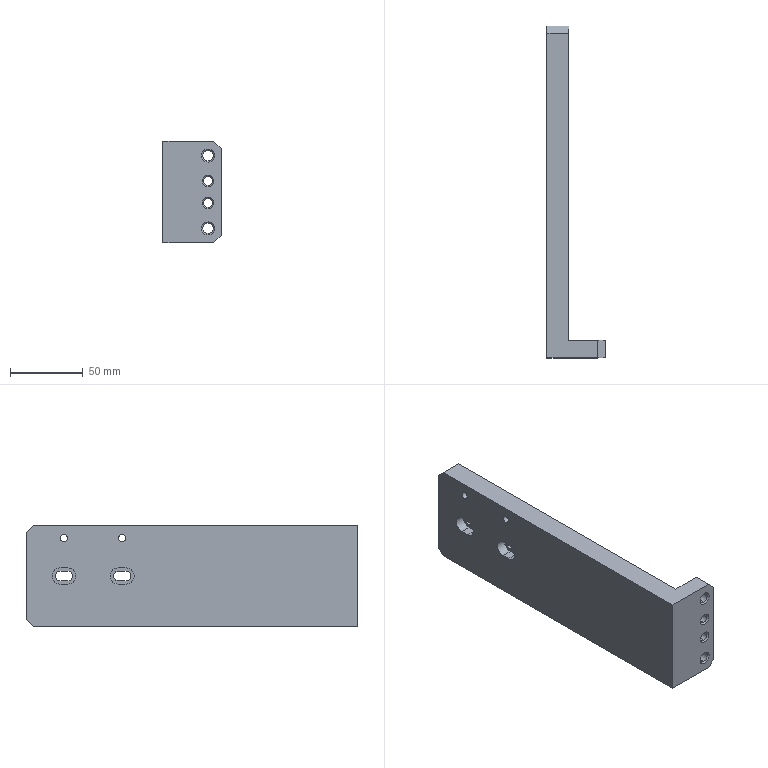Part | SolidWorks | features HoleWzd 3, Chamfer 2, ICE 2, Cut 1, Extrusion 1 | 1 solid | 78 faces | box 40 x 228 x 70 mm | volume 254196 mm3 | plane 38 | cone 20 | cylinder 20 | commonest cylinder face diameters 5 x4 6 x4 6.6 x4 7 x4 11 x4